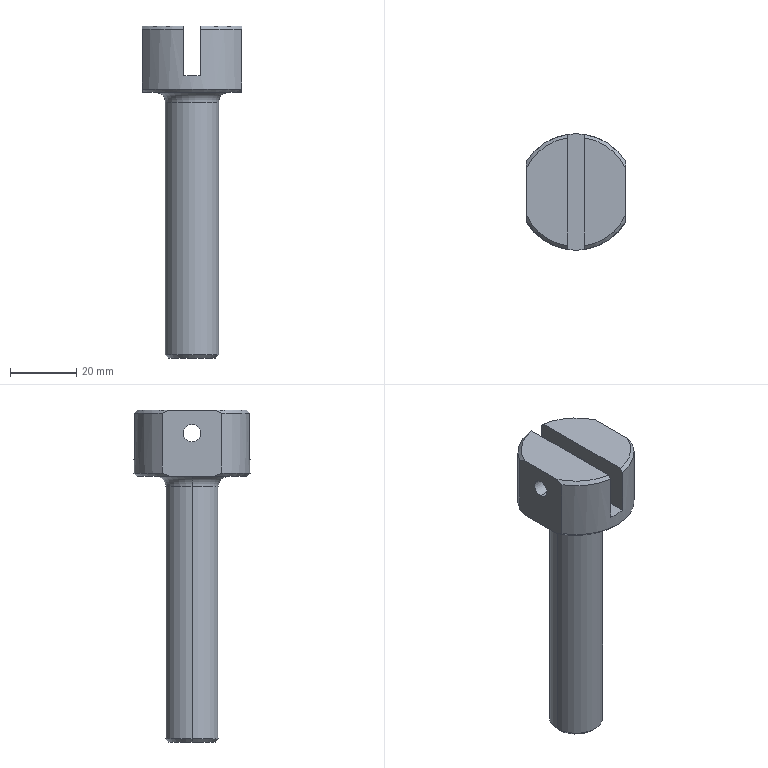Part | SolidWorks | features BaseBody 1 | 1 solid | 27 faces | box 30 x 35 x 100 mm | volume 30973 mm3 | plane 9 | cylinder 8 | cone 8 | torus 2 | commonest cylinder face diameters 5.2 x4 16 x2 35 x2
STEP:
#1=CARTESIAN_POINT('',(-2.5,0.,95.6));
#2=VERTEX_POINT('',#1);
#3=CARTESIAN_POINT('',(-2.5,0.,90.4));
#4=VERTEX_POINT('',#3);
#5=CARTESIAN_POINT('',(-2.5,0.,93.));
#6=DIRECTION('',(1.,0.,0.));
#7=DIRECTION('',(0.,-1.,0.));
#8=AXIS2_PLACEMENT_3D('',#5,#6,#7);
#9=CIRCLE('',#8,2.6);
#10=EDGE_CURVE('',#2,#4,#9,.T.);
#11=ORIENTED_EDGE('',*,*,#10,.T.);
#12=CARTESIAN_POINT('',(-15.,0.,90.4));
#13=VERTEX_POINT('',#12);
#14=CARTESIAN_POINT('',(-15.,0.,90.4));
#15=DIRECTION('',(-1.,0.,0.));
#16=VECTOR('',#15,1000.);
#17=LINE('',#14,#16);
#18=EDGE_CURVE('',#4,#13,#17,.T.);
#19=ORIENTED_EDGE('',*,*,#18,.T.);
#20=CARTESIAN_POINT('',(-15.,0.,95.6));
#21=VERTEX_POINT('',#20);
#22=CARTESIAN_POINT('',(-15.,0.,93.));
#23=DIRECTION('',(-1.,0.,0.));
#24=DIRECTION('',(0.,0.,1.));
#25=AXIS2_PLACEMENT_3D('',#22,#23,#24);
#26=CIRCLE('',#25,2.6);
#27=EDGE_CURVE('',#13,#21,#26,.T.);
#28=ORIENTED_EDGE('',*,*,#27,.T.);
#29=CARTESIAN_POINT('',(-15.,0.,95.6));
#30=DIRECTION('',(-1.,0.,0.));
#31=VECTOR('',#30,1000.);
#32=LINE('',#29,#31);
#33=EDGE_CURVE('',#2,#21,#32,.T.);
#34=ORIENTED_EDGE('',*,*,#33,.F.);
#35=EDGE_LOOP('',(#11,#19,#28,#34));
#36=FACE_OUTER_BOUND('',#35,.T.);
#37=CARTESIAN_POINT('',(-15.,0.,93.));
#38=DIRECTION('',(-1.,0.,0.));
#39=DIRECTION('',(0.,0.,1.));
#40=AXIS2_PLACEMENT_3D('',#37,#38,#39);
#41=CYLINDRICAL_SURFACE('',#40,2.6);
#42=ADVANCED_FACE('',(#36),#41,.F.);
#43=CARTESIAN_POINT('',(-7.,0.,0.));
#44=VERTEX_POINT('',#43);
#45=CARTESIAN_POINT('',(7.,0.,0.));
#46=VERTEX_POINT('',#45);
#47=CARTESIAN_POINT('',(0.,0.,0.));
#48=DIRECTION('',(0.,0.,-1.));
#49=DIRECTION('',(1.,0.,0.));
#50=AXIS2_PLACEMENT_3D('',#47,#48,#49);
#51=CIRCLE('',#50,7.);
#52=EDGE_CURVE('',#44,#46,#51,.T.);
#53=ORIENTED_EDGE('',*,*,#52,.F.);
#54=CARTESIAN_POINT('',(-8.,0.,1.));
#55=VERTEX_POINT('',#54);
#56=CARTESIAN_POINT('',(-8.,0.,1.));
#57=DIRECTION('',(-0.7071,0.,0.7071));
#58=VECTOR('',#57,1000.);
#59=LINE('',#56,#58);
#60=EDGE_CURVE('',#44,#55,#59,.T.);
#61=ORIENTED_EDGE('',*,*,#60,.T.);
#62=CARTESIAN_POINT('',(8.,0.,1.));
#63=VERTEX_POINT('',#62);
#64=CARTESIAN_POINT('',(0.,0.,1.));
#65=DIRECTION('',(0.,0.,1.));
#66=DIRECTION('',(1.,0.,0.));
#67=AXIS2_PLACEMENT_3D('',#64,#65,#66);
#68=CIRCLE('',#67,8.);
#69=EDGE_CURVE('',#63,#55,#68,.T.);
#70=ORIENTED_EDGE('',*,*,#69,.F.);
#71=CARTESIAN_POINT('',(8.,0.,1.));
#72=DIRECTION('',(0.7071,0.,0.7071));
#73=VECTOR('',#72,1000.);
#74=LINE('',#71,#73);
#75=EDGE_CURVE('',#46,#63,#74,.T.);
#76=ORIENTED_EDGE('',*,*,#75,.F.);
#77=EDGE_LOOP('',(#53,#61,#70,#76));
#78=FACE_OUTER_BOUND('',#77,.T.);
#79=CARTESIAN_POINT('',(0.,0.,1.));
#80=DIRECTION('',(0.,0.,1.));
#81=DIRECTION('',(1.,0.,0.));
#82=AXIS2_PLACEMENT_3D('',#79,#80,#81);
#83=CONICAL_SURFACE('',#82,8.,0.7854);
#84=ADVANCED_FACE('',(#78),#83,.T.);
#85=CARTESIAN_POINT('',(-11.,0.,80.));
#86=VERTEX_POINT('',#85);
#87=CARTESIAN_POINT('',(11.,0.,80.));
#88=VERTEX_POINT('',#87);
#89=CARTESIAN_POINT('',(0.,0.,80.));
#90=DIRECTION('',(0.,0.,1.));
#91=DIRECTION('',(1.,0.,0.));
#92=AXIS2_PLACEMENT_3D('',#89,#90,#91);
#93=CIRCLE('',#92,11.);
#94=EDGE_CURVE('',#86,#88,#93,.T.);
#95=ORIENTED_EDGE('',*,*,#94,.F.);
#96=CARTESIAN_POINT('',(-8.,0.,77.));
#97=VERTEX_POINT('',#96);
#98=CARTESIAN_POINT('',(-11.,0.,77.));
#99=DIRECTION('',(0.,1.,0.));
#100=DIRECTION('',(-1.,0.,0.));
#101=AXIS2_PLACEMENT_3D('',#98,#99,#100);
#102=CIRCLE('',#101,3.);
#103=EDGE_CURVE('',#86,#97,#102,.T.);
#104=ORIENTED_EDGE('',*,*,#103,.T.);
#105=CARTESIAN_POINT('',(8.,0.,77.));
#106=VERTEX_POINT('',#105);
#107=CARTESIAN_POINT('',(0.,0.,77.));
#108=DIRECTION('',(0.,0.,-1.));
#109=DIRECTION('',(1.,0.,0.));
#110=AXIS2_PLACEMENT_3D('',#107,#108,#109);
#111=CIRCLE('',#110,8.);
#112=EDGE_CURVE('',#106,#97,#111,.T.);
#113=ORIENTED_EDGE('',*,*,#112,.F.);
#114=CARTESIAN_POINT('',(11.,0.,77.));
#115=DIRECTION('',(0.,-1.,0.));
#116=DIRECTION('',(0.,0.,-1.));
#117=AXIS2_PLACEMENT_3D('',#114,#115,#116);
#118=CIRCLE('',#117,3.);
#119=EDGE_CURVE('',#88,#106,#118,.T.);
#120=ORIENTED_EDGE('',*,*,#119,.F.);
#121=EDGE_LOOP('',(#95,#104,#113,#120));
#122=FACE_OUTER_BOUND('',#121,.T.);
#123=CARTESIAN_POINT('',(0.,0.,77.));
#124=DIRECTION('',(0.,0.,1.));
#125=DIRECTION('',(1.,0.,0.));
#126=AXIS2_PLACEMENT_3D('',#123,#124,#125);
#127=TOROIDAL_SURFACE('',#126,11.,3.);
#128=ADVANCED_FACE('',(#122),#127,.F.);
#129=CARTESIAN_POINT('',(0.,0.,77.));
#130=DIRECTION('',(0.,0.,-1.));
#131=DIRECTION('',(1.,0.,0.));
#132=AXIS2_PLACEMENT_3D('',#129,#130,#131);
#133=CIRCLE('',#132,8.);
#134=EDGE_CURVE('',#97,#106,#133,.T.);
#135=ORIENTED_EDGE('',*,*,#134,.T.);
#136=CARTESIAN_POINT('',(8.,0.,80.));
#137=DIRECTION('',(0.,0.,-1.));
#138=VECTOR('',#137,1000.);
#139=LINE('',#136,#138);
#140=EDGE_CURVE('',#106,#63,#139,.T.);
#141=ORIENTED_EDGE('',*,*,#140,.T.);
#142=ORIENTED_EDGE('',*,*,#69,.T.);
#143=CARTESIAN_POINT('',(-8.,0.,80.));
#144=DIRECTION('',(0.,0.,-1.));
#145=VECTOR('',#144,1000.);
#146=LINE('',#143,#145);
#147=EDGE_CURVE('',#97,#55,#146,.T.);
#148=ORIENTED_EDGE('',*,*,#147,.F.);
#149=EDGE_LOOP('',(#135,#141,#142,#148));
#150=FACE_OUTER_BOUND('',#149,.T.);
#151=CARTESIAN_POINT('',(0.,0.,80.));
#152=DIRECTION('',(0.,0.,-1.));
#153=DIRECTION('',(-1.,0.,0.));
#154=AXIS2_PLACEMENT_3D('',#151,#152,#153);
#155=CYLINDRICAL_SURFACE('',#154,8.);
#156=ADVANCED_FACE('',(#150),#155,.T.);
#157=CARTESIAN_POINT('',(15.,0.,90.4));
#158=VERTEX_POINT('',#157);
#159=CARTESIAN_POINT('',(15.,0.,95.6));
#160=VERTEX_POINT('',#159);
#161=CARTESIAN_POINT('',(15.,0.,93.));
#162=DIRECTION('',(-1.,0.,0.));
#163=DIRECTION('',(0.,0.,1.));
#164=AXIS2_PLACEMENT_3D('',#161,#162,#163);
#165=CIRCLE('',#164,2.6);
#166=EDGE_CURVE('',#158,#160,#165,.T.);
#167=ORIENTED_EDGE('',*,*,#166,.F.);
#168=CARTESIAN_POINT('',(2.5,0.,90.4));
#169=VERTEX_POINT('',#168);
#170=CARTESIAN_POINT('',(-15.,0.,90.4));
#171=DIRECTION('',(-1.,0.,0.));
#172=VECTOR('',#171,1000.);
#173=LINE('',#170,#172);
#174=EDGE_CURVE('',#158,#169,#173,.T.);
#175=ORIENTED_EDGE('',*,*,#174,.T.);
#176=CARTESIAN_POINT('',(2.5,0.,95.6));
#177=VERTEX_POINT('',#176);
#178=CARTESIAN_POINT('',(2.5,0.,93.));
#179=DIRECTION('',(-1.,0.,0.));
#180=DIRECTION('',(0.,1.,0.));
#181=AXIS2_PLACEMENT_3D('',#178,#179,#180);
#182=CIRCLE('',#181,2.6);
#183=EDGE_CURVE('',#169,#177,#182,.T.);
#184=ORIENTED_EDGE('',*,*,#183,.T.);
#185=CARTESIAN_POINT('',(-15.,0.,95.6));
#186=DIRECTION('',(-1.,0.,0.));
#187=VECTOR('',#186,1000.);
#188=LINE('',#185,#187);
#189=EDGE_CURVE('',#160,#177,#188,.T.);
#190=ORIENTED_EDGE('',*,*,#189,.F.);
#191=EDGE_LOOP('',(#167,#175,#184,#190));
#192=FACE_OUTER_BOUND('',#191,.T.);
#193=CARTESIAN_POINT('',(-15.,0.,93.));
#194=DIRECTION('',(-1.,0.,0.));
#195=DIRECTION('',(0.,0.,1.));
#196=AXIS2_PLACEMENT_3D('',#193,#194,#195);
#197=CYLINDRICAL_SURFACE('',#196,2.6);
#198=ADVANCED_FACE('',(#192),#197,.F.);
#199=CARTESIAN_POINT('',(2.5,16.31,100.));
#200=VERTEX_POINT('',#199);
#201=CARTESIAN_POINT('',(2.5,17.321,99.));
#202=VERTEX_POINT('',#201);
#203=CARTESIAN_POINT('',(2.5,16.31,100.));
#204=CARTESIAN_POINT('',(2.5,16.647,99.667));
#205=CARTESIAN_POINT('',(2.5,16.984,99.333));
#206=CARTESIAN_POINT('',(2.5,17.321,99.));
#207=B_SPLINE_CURVE_WITH_KNOTS('',3,(#203,#204,#205,#206),.UNSPECIFIED.,.F.,.F.,(4,4),(0.01912,0.02054),.UNSPECIFIED.);
#208=EDGE_CURVE('',#200,#202,#207,.T.);
#209=ORIENTED_EDGE('',*,*,#208,.F.);
#210=CARTESIAN_POINT('',(15.,6.874,100.));
#211=VERTEX_POINT('',#210);
#212=CARTESIAN_POINT('',(0.,0.,100.));
#213=DIRECTION('',(0.,0.,1.));
#214=DIRECTION('',(1.,0.,0.));
#215=AXIS2_PLACEMENT_3D('',#212,#213,#214);
#216=CIRCLE('',#215,16.5);
#217=EDGE_CURVE('',#211,#200,#216,.T.);
#218=ORIENTED_EDGE('',*,*,#217,.F.);
#219=CARTESIAN_POINT('',(15.,9.014,99.));
#220=VERTEX_POINT('',#219);
#221=CARTESIAN_POINT('',(15.,9.014,99.));
#222=CARTESIAN_POINT('',(15.,8.312,99.362));
#223=CARTESIAN_POINT('',(15.,7.599,99.698));
#224=CARTESIAN_POINT('',(15.,6.874,100.));
#225=B_SPLINE_CURVE_WITH_KNOTS('',3,(#221,#222,#223,#224),.UNSPECIFIED.,.F.,.F.,(4,4),(0.01311,0.01546),.UNSPECIFIED.);
#226=EDGE_CURVE('',#220,#211,#225,.T.);
#227=ORIENTED_EDGE('',*,*,#226,.F.);
#228=CARTESIAN_POINT('',(0.,0.,99.));
#229=DIRECTION('',(0.,0.,-1.));
#230=DIRECTION('',(1.,0.,0.));
#231=AXIS2_PLACEMENT_3D('',#228,#229,#230);
#232=CIRCLE('',#231,17.5);
#233=EDGE_CURVE('',#202,#220,#232,.T.);
#234=ORIENTED_EDGE('',*,*,#233,.F.);
#235=EDGE_LOOP('',(#209,#218,#227,#234));
#236=FACE_OUTER_BOUND('',#235,.T.);
#237=CARTESIAN_POINT('',(0.,0.,100.));
#238=DIRECTION('',(0.,0.,-1.));
#239=DIRECTION('',(-1.,0.,0.));
#240=AXIS2_PLACEMENT_3D('',#237,#238,#239);
#241=CONICAL_SURFACE('',#240,16.5,0.7854);
#242=ADVANCED_FACE('',(#236),#241,.T.);
#243=CARTESIAN_POINT('',(2.5,-16.31,100.));
#244=VERTEX_POINT('',#243);
#245=CARTESIAN_POINT('',(2.5,21.611,100.));
#246=DIRECTION('',(0.,1.,0.));
#247=VECTOR('',#246,1000.);
#248=LINE('',#245,#247);
#249=EDGE_CURVE('',#244,#200,#248,.T.);
#250=ORIENTED_EDGE('',*,*,#249,.F.);
#251=CARTESIAN_POINT('',(15.,-6.874,100.));
#252=VERTEX_POINT('',#251);
#253=CARTESIAN_POINT('',(0.,0.,100.));
#254=DIRECTION('',(0.,0.,1.));
#255=DIRECTION('',(1.,0.,0.));
#256=AXIS2_PLACEMENT_3D('',#253,#254,#255);
#257=CIRCLE('',#256,16.5);
#258=EDGE_CURVE('',#244,#252,#257,.T.);
#259=ORIENTED_EDGE('',*,*,#258,.T.);
#260=CARTESIAN_POINT('',(15.,9.014,100.));
#261=DIRECTION('',(0.,-1.,0.));
#262=VECTOR('',#261,1000.);
#263=LINE('',#260,#262);
#264=EDGE_CURVE('',#211,#252,#263,.T.);
#265=ORIENTED_EDGE('',*,*,#264,.F.);
#266=ORIENTED_EDGE('',*,*,#217,.T.);
#267=EDGE_LOOP('',(#250,#259,#265,#266));
#268=FACE_OUTER_BOUND('',#267,.T.);
#269=CARTESIAN_POINT('',(0.,0.,100.));
#270=DIRECTION('',(0.,0.,1.));
#271=DIRECTION('',(1.,0.,0.));
#272=AXIS2_PLACEMENT_3D('',#269,#270,#271);
#273=PLANE('',#272);
#274=ADVANCED_FACE('',(#268),#273,.T.);
#275=CARTESIAN_POINT('',(2.5,-17.321,99.));
#276=VERTEX_POINT('',#275);
#277=CARTESIAN_POINT('',(2.5,-17.321,99.));
#278=CARTESIAN_POINT('',(2.5,-16.984,99.333));
#279=CARTESIAN_POINT('',(2.5,-16.647,99.667));
#280=CARTESIAN_POINT('',(2.5,-16.31,100.));
#281=B_SPLINE_CURVE_WITH_KNOTS('',3,(#277,#278,#279,#280),.UNSPECIFIED.,.F.,.F.,(4,4),(0.01819,0.01961),.UNSPECIFIED.);
#282=EDGE_CURVE('',#276,#244,#281,.T.);
#283=ORIENTED_EDGE('',*,*,#282,.F.);
#284=CARTESIAN_POINT('',(15.,-9.014,99.));
#285=VERTEX_POINT('',#284);
#286=CARTESIAN_POINT('',(0.,0.,99.));
#287=DIRECTION('',(0.,0.,-1.));
#288=DIRECTION('',(1.,0.,0.));
#289=AXIS2_PLACEMENT_3D('',#286,#287,#288);
#290=CIRCLE('',#289,17.5);
#291=EDGE_CURVE('',#285,#276,#290,.T.);
#292=ORIENTED_EDGE('',*,*,#291,.F.);
#293=CARTESIAN_POINT('',(15.,-6.874,100.));
#294=CARTESIAN_POINT('',(15.,-7.598,99.698));
#295=CARTESIAN_POINT('',(15.,-8.313,99.361));
#296=CARTESIAN_POINT('',(15.,-9.014,99.));
#297=B_SPLINE_CURVE_WITH_KNOTS('',3,(#293,#294,#295,#296),.UNSPECIFIED.,.F.,.F.,(4,4),(0.02959,0.03195),.UNSPECIFIED.);
#298=EDGE_CURVE('',#252,#285,#297,.T.);
#299=ORIENTED_EDGE('',*,*,#298,.F.);
#300=ORIENTED_EDGE('',*,*,#258,.F.);
#301=EDGE_LOOP('',(#283,#292,#299,#300));
#302=FACE_OUTER_BOUND('',#301,.T.);
#303=CARTESIAN_POINT('',(0.,0.,100.));
#304=DIRECTION('',(0.,0.,-1.));
#305=DIRECTION('',(-1.,0.,0.));
#306=AXIS2_PLACEMENT_3D('',#303,#304,#305);
#307=CONICAL_SURFACE('',#306,16.5,0.7854);
#308=ADVANCED_FACE('',(#302),#307,.T.);
#309=ORIENTED_EDGE('',*,*,#174,.F.);
#310=CARTESIAN_POINT('',(15.,0.,93.));
#311=DIRECTION('',(-1.,0.,0.));
#312=DIRECTION('',(0.,0.,1.));
#313=AXIS2_PLACEMENT_3D('',#310,#311,#312);
#314=CIRCLE('',#313,2.6);
#315=EDGE_CURVE('',#160,#158,#314,.T.);
#316=ORIENTED_EDGE('',*,*,#315,.F.);
#317=ORIENTED_EDGE('',*,*,#189,.T.);
#318=CARTESIAN_POINT('',(2.5,0.,93.));
#319=DIRECTION('',(-1.,0.,0.));
#320=DIRECTION('',(0.,1.,0.));
#321=AXIS2_PLACEMENT_3D('',#318,#319,#320);
#322=CIRCLE('',#321,2.6);
#323=EDGE_CURVE('',#177,#169,#322,.T.);
#324=ORIENTED_EDGE('',*,*,#323,.T.);
#325=EDGE_LOOP('',(#309,#316,#317,#324));
#326=FACE_OUTER_BOUND('',#325,.T.);
#327=CARTESIAN_POINT('',(-15.,0.,93.));
#328=DIRECTION('',(-1.,0.,0.));
#329=DIRECTION('',(0.,0.,1.));
#330=AXIS2_PLACEMENT_3D('',#327,#328,#329);
#331=CYLINDRICAL_SURFACE('',#330,2.6);
#332=ADVANCED_FACE('',(#326),#331,.F.);
#333=CARTESIAN_POINT('',(-15.,-9.014,99.));
#334=VERTEX_POINT('',#333);
#335=CARTESIAN_POINT('',(-15.,-6.874,100.));
#336=VERTEX_POINT('',#335);
#337=CARTESIAN_POINT('',(-15.,-9.014,99.));
#338=CARTESIAN_POINT('',(-15.,-8.312,99.362));
#339=CARTESIAN_POINT('',(-15.,-7.599,99.698));
#340=CARTESIAN_POINT('',(-15.,-6.874,100.));
#341=B_SPLINE_CURVE_WITH_KNOTS('',3,(#337,#338,#339,#340),.UNSPECIFIED.,.F.,.F.,(4,4),(0.01311,0.01546),.UNSPECIFIED.);
#342=EDGE_CURVE('',#334,#336,#341,.T.);
#343=ORIENTED_EDGE('',*,*,#342,.T.);
#344=CARTESIAN_POINT('',(-15.,6.874,100.));
#345=VERTEX_POINT('',#344);
#346=CARTESIAN_POINT('',(-15.,9.014,100.));
#347=DIRECTION('',(0.,1.,0.));
#348=VECTOR('',#347,1000.);
#349=LINE('',#346,#348);
#350=EDGE_CURVE('',#336,#345,#349,.T.);
#351=ORIENTED_EDGE('',*,*,#350,.T.);
#352=CARTESIAN_POINT('',(-15.,9.014,99.));
#353=VERTEX_POINT('',#352);
#354=CARTESIAN_POINT('',(-15.,6.874,100.));
#355=CARTESIAN_POINT('',(-15.,7.598,99.698));
#356=CARTESIAN_POINT('',(-15.,8.313,99.361));
#357=CARTESIAN_POINT('',(-15.,9.014,99.));
#358=B_SPLINE_CURVE_WITH_KNOTS('',3,(#354,#355,#356,#357),.UNSPECIFIED.,.F.,.F.,(4,4),(0.02959,0.03195),.UNSPECIFIED.);
#359=EDGE_CURVE('',#345,#353,#358,.T.);
#360=ORIENTED_EDGE('',*,*,#359,.T.);
#361=CARTESIAN_POINT('',(-15.,9.014,81.));
#362=VERTEX_POINT('',#361);
#363=CARTESIAN_POINT('',(-15.,9.014,80.));
#364=DIRECTION('',(0.,0.,1.));
#365=VECTOR('',#364,1000.);
#366=LINE('',#363,#365);
#367=EDGE_CURVE('',#362,#353,#366,.T.);
#368=ORIENTED_EDGE('',*,*,#367,.F.);
#369=CARTESIAN_POINT('',(-15.,6.874,80.));
#370=VERTEX_POINT('',#369);
#371=CARTESIAN_POINT('',(-15.,9.014,81.));
#372=CARTESIAN_POINT('',(-15.,8.312,80.638));
#373=CARTESIAN_POINT('',(-15.,7.599,80.302));
#374=CARTESIAN_POINT('',(-15.,6.874,80.));
#375=B_SPLINE_CURVE_WITH_KNOTS('',3,(#371,#372,#373,#374),.UNSPECIFIED.,.F.,.F.,(4,4),(0.01311,0.01546),.UNSPECIFIED.);
#376=EDGE_CURVE('',#362,#370,#375,.T.);
#377=ORIENTED_EDGE('',*,*,#376,.T.);
#378=CARTESIAN_POINT('',(-15.,-6.874,80.));
#379=VERTEX_POINT('',#378);
#380=CARTESIAN_POINT('',(-15.,9.014,80.));
#381=DIRECTION('',(0.,1.,0.));
#382=VECTOR('',#381,1000.);
#383=LINE('',#380,#382);
#384=EDGE_CURVE('',#379,#370,#383,.T.);
#385=ORIENTED_EDGE('',*,*,#384,.F.);
#386=CARTESIAN_POINT('',(-15.,-9.014,81.));
#387=VERTEX_POINT('',#386);
#388=CARTESIAN_POINT('',(-15.,-6.874,80.));
#389=CARTESIAN_POINT('',(-15.,-7.598,80.302));
#390=CARTESIAN_POINT('',(-15.,-8.313,80.639));
#391=CARTESIAN_POINT('',(-15.,-9.014,81.));
#392=B_SPLINE_CURVE_WITH_KNOTS('',3,(#388,#389,#390,#391),.UNSPECIFIED.,.F.,.F.,(4,4),(0.02959,0.03195),.UNSPECIFIED.);
#393=EDGE_CURVE('',#379,#387,#392,.T.);
#394=ORIENTED_EDGE('',*,*,#393,.T.);
#395=CARTESIAN_POINT('',(-15.,-9.014,80.));
#396=DIRECTION('',(0.,0.,1.));
#397=VECTOR('',#396,1000.);
#398=LINE('',#395,#397);
#399=EDGE_CURVE('',#387,#334,#398,.T.);
#400=ORIENTED_EDGE('',*,*,#399,.T.);
#401=EDGE_LOOP('',(#343,#351,#360,#368,#377,#385,#394,#400));
#402=FACE_OUTER_BOUND('',#401,.T.);
#403=CARTESIAN_POINT('',(-15.,0.,93.));
#404=DIRECTION('',(-1.,0.,0.));
#405=DIRECTION('',(0.,0.,1.));
#406=AXIS2_PLACEMENT_3D('',#403,#404,#405);
#407=CIRCLE('',#406,2.6);
#408=EDGE_CURVE('',#21,#13,#407,.T.);
#409=ORIENTED_EDGE('',*,*,#408,.F.);
#410=ORIENTED_EDGE('',*,*,#27,.F.);
#411=EDGE_LOOP('',(#409,#410));
#412=FACE_BOUND('',#411,.T.);
#413=CARTESIAN_POINT('',(-15.,9.014,80.));
#414=DIRECTION('',(1.,0.,0.));
#415=DIRECTION('',(0.,0.,-1.));
#416=AXIS2_PLACEMENT_3D('',#413,#414,#415);
#417=PLANE('',#416);
#418=ADVANCED_FACE('',(#402,#412),#417,.F.);
#419=CARTESIAN_POINT('',(2.5,17.321,85.));
#420=VERTEX_POINT('',#419);
#421=CARTESIAN_POINT('',(-2.5,17.321,85.));
#422=VERTEX_POINT('',#421);
#423=CARTESIAN_POINT('',(0.,0.,85.));
#424=DIRECTION('',(0.,0.,1.));
#425=DIRECTION('',(1.,0.,0.));
#426=AXIS2_PLACEMENT_3D('',#423,#424,#425);
#427=CIRCLE('',#426,17.5);
#428=EDGE_CURVE('',#420,#422,#427,.T.);
#429=ORIENTED_EDGE('',*,*,#428,.F.);
#430=CARTESIAN_POINT('',(2.5,17.321,100.));
#431=DIRECTION('',(0.,0.,1.));
#432=VECTOR('',#431,1000.);
#433=LINE('',#430,#432);
#434=EDGE_CURVE('',#420,#202,#433,.T.);
#435=ORIENTED_EDGE('',*,*,#434,.T.);
#436=ORIENTED_EDGE('',*,*,#233,.T.);
#437=CARTESIAN_POINT('',(15.,9.014,81.));
#438=VERTEX_POINT('',#437);
#439=CARTESIAN_POINT('',(15.,9.014,80.));
#440=DIRECTION('',(0.,0.,1.));
#441=VECTOR('',#440,1000.);
#442=LINE('',#439,#441);
#443=EDGE_CURVE('',#438,#220,#442,.T.);
#444=ORIENTED_EDGE('',*,*,#443,.F.);
#445=CARTESIAN_POINT('',(0.,0.,81.));
#446=DIRECTION('',(0.,0.,1.));
#447=DIRECTION('',(1.,0.,0.));
#448=AXIS2_PLACEMENT_3D('',#445,#446,#447);
#449=CIRCLE('',#448,17.5);
#450=EDGE_CURVE('',#438,#362,#449,.T.);
#451=ORIENTED_EDGE('',*,*,#450,.T.);
#452=ORIENTED_EDGE('',*,*,#367,.T.);
#453=CARTESIAN_POINT('',(-2.5,17.321,99.));
#454=VERTEX_POINT('',#453);
#455=CARTESIAN_POINT('',(0.,0.,99.));
#456=DIRECTION('',(0.,0.,-1.));
#457=DIRECTION('',(1.,0.,0.));
#458=AXIS2_PLACEMENT_3D('',#455,#456,#457);
#459=CIRCLE('',#458,17.5);
#460=EDGE_CURVE('',#353,#454,#459,.T.);
#461=ORIENTED_EDGE('',*,*,#460,.T.);
#462=CARTESIAN_POINT('',(-2.5,17.321,100.));
#463=DIRECTION('',(0.,0.,-1.));
#464=VECTOR('',#463,1000.);
#465=LINE('',#462,#464);
#466=EDGE_CURVE('',#454,#422,#465,.T.);
#467=ORIENTED_EDGE('',*,*,#466,.T.);
#468=EDGE_LOOP('',(#429,#435,#436,#444,#451,#452,#461,#467));
#469=FACE_OUTER_BOUND('',#468,.T.);
#470=CARTESIAN_POINT('',(0.,0.,100.));
#471=DIRECTION('',(0.,0.,-1.));
#472=DIRECTION('',(-1.,0.,0.));
#473=AXIS2_PLACEMENT_3D('',#470,#471,#472);
#474=CYLINDRICAL_SURFACE('',#473,17.5);
#475=ADVANCED_FACE('',(#469),#474,.T.);
#476=CARTESIAN_POINT('',(-2.5,16.31,100.));
#477=VERTEX_POINT('',#476);
#478=CARTESIAN_POINT('',(-2.5,17.321,99.));
#479=CARTESIAN_POINT('',(-2.5,16.984,99.333));
#480=CARTESIAN_POINT('',(-2.5,16.647,99.667));
#481=CARTESIAN_POINT('',(-2.5,16.31,100.));
#482=B_SPLINE_CURVE_WITH_KNOTS('',3,(#478,#479,#480,#481),.UNSPECIFIED.,.F.,.F.,(4,4),(0.01819,0.01961),.UNSPECIFIED.);
#483=EDGE_CURVE('',#454,#477,#482,.T.);
#484=ORIENTED_EDGE('',*,*,#483,.F.);
#485=ORIENTED_EDGE('',*,*,#460,.F.);
#486=ORIENTED_EDGE('',*,*,#359,.F.);
#487=CARTESIAN_POINT('',(0.,0.,100.));
#488=DIRECTION('',(0.,0.,1.));
#489=DIRECTION('',(1.,0.,0.));
#490=AXIS2_PLACEMENT_3D('',#487,#488,#489);
#491=CIRCLE('',#490,16.5);
#492=EDGE_CURVE('',#477,#345,#491,.T.);
#493=ORIENTED_EDGE('',*,*,#492,.F.);
#494=EDGE_LOOP('',(#484,#485,#486,#493));
#495=FACE_OUTER_BOUND('',#494,.T.);
#496=CARTESIAN_POINT('',(0.,0.,100.));
#497=DIRECTION('',(0.,0.,-1.));
#498=DIRECTION('',(-1.,0.,0.));
#499=AXIS2_PLACEMENT_3D('',#496,#497,#498);
#500=CONICAL_SURFACE('',#499,16.5,0.7854);
#501=ADVANCED_FACE('',(#495),#500,.T.);
#502=CARTESIAN_POINT('',(15.,-9.014,81.));
#503=VERTEX_POINT('',#502);
#504=CARTESIAN_POINT('',(15.,-6.874,80.));
#505=VERTEX_POINT('',#504);
#506=CARTESIAN_POINT('',(15.,-9.014,81.));
#507=CARTESIAN_POINT('',(15.,-8.312,80.638));
#508=CARTESIAN_POINT('',(15.,-7.599,80.302));
#509=CARTESIAN_POINT('',(15.,-6.874,80.));
#510=B_SPLINE_CURVE_WITH_KNOTS('',3,(#506,#507,#508,#509),.UNSPECIFIED.,.F.,.F.,(4,4),(0.01311,0.01546),.UNSPECIFIED.);
#511=EDGE_CURVE('',#503,#505,#510,.T.);
#512=ORIENTED_EDGE('',*,*,#511,.F.);
#513=CARTESIAN_POINT('',(0.,0.,81.));
#514=DIRECTION('',(0.,0.,1.));
#515=DIRECTION('',(1.,0.,0.));
#516=AXIS2_PLACEMENT_3D('',#513,#514,#515);
#517=CIRCLE('',#516,17.5);
#518=EDGE_CURVE('',#387,#503,#517,.T.);
#519=ORIENTED_EDGE('',*,*,#518,.F.);
#520=ORIENTED_EDGE('',*,*,#393,.F.);
#521=CARTESIAN_POINT('',(0.,0.,80.));
#522=DIRECTION('',(0.,0.,-1.));
#523=DIRECTION('',(1.,0.,0.));
#524=AXIS2_PLACEMENT_3D('',#521,#522,#523);
#525=CIRCLE('',#524,16.5);
#526=EDGE_CURVE('',#505,#379,#525,.T.);
#527=ORIENTED_EDGE('',*,*,#526,.F.);
#528=EDGE_LOOP('',(#512,#519,#520,#527));
#529=FACE_OUTER_BOUND('',#528,.T.);
#530=CARTESIAN_POINT('',(0.,0.,81.));
#531=DIRECTION('',(0.,0.,1.));
#532=DIRECTION('',(1.,0.,0.));
#533=AXIS2_PLACEMENT_3D('',#530,#531,#532);
#534=CONICAL_SURFACE('',#533,17.5,0.7854);
#535=ADVANCED_FACE('',(#529),#534,.T.);
#536=ORIENTED_EDGE('',*,*,#140,.F.);
#537=ORIENTED_EDGE('',*,*,#112,.T.);
#538=ORIENTED_EDGE('',*,*,#147,.T.);
#539=CARTESIAN_POINT('',(0.,0.,1.));
#540=DIRECTION('',(0.,0.,1.));
#541=DIRECTION('',(1.,0.,0.));
#542=AXIS2_PLACEMENT_3D('',#539,#540,#541);
#543=CIRCLE('',#542,8.);
#544=EDGE_CURVE('',#55,#63,#543,.T.);
#545=ORIENTED_EDGE('',*,*,#544,.T.);
#546=EDGE_LOOP('',(#536,#537,#538,#545));
#547=FACE_OUTER_BOUND('',#546,.T.);
#548=CARTESIAN_POINT('',(0.,0.,80.));
#549=DIRECTION('',(0.,0.,-1.));
#550=DIRECTION('',(-1.,0.,0.));
#551=AXIS2_PLACEMENT_3D('',#548,#549,#550);
#552=CYLINDRICAL_SURFACE('',#551,8.);
#553=ADVANCED_FACE('',(#547),#552,.T.);
#554=CARTESIAN_POINT('',(0.,0.,0.));
#555=DIRECTION('',(0.,0.,-1.));
#556=DIRECTION('',(1.,0.,0.));
#557=AXIS2_PLACEMENT_3D('',#554,#555,#556);
#558=CIRCLE('',#557,7.);
#559=EDGE_CURVE('',#46,#44,#558,.T.);
#560=ORIENTED_EDGE('',*,*,#559,.T.);
#561=ORIENTED_EDGE('',*,*,#52,.T.);
#562=EDGE_LOOP('',(#560,#561));
#563=FACE_OUTER_BOUND('',#562,.T.);
#564=CARTESIAN_POINT('',(0.,0.,0.));
#565=DIRECTION('',(0.,0.,1.));
#566=DIRECTION('',(1.,0.,0.));
#567=AXIS2_PLACEMENT_3D('',#564,#565,#566);
#568=PLANE('',#567);
#569=ADVANCED_FACE('',(#563),#568,.F.);
#570=ORIENTED_EDGE('',*,*,#291,.T.);
#571=CARTESIAN_POINT('',(2.5,-17.321,85.));
#572=VERTEX_POINT('',#571);
#573=CARTESIAN_POINT('',(2.5,-17.321,100.));
#574=DIRECTION('',(0.,0.,-1.));
#575=VECTOR('',#574,1000.);
#576=LINE('',#573,#575);
#577=EDGE_CURVE('',#276,#572,#576,.T.);
#578=ORIENTED_EDGE('',*,*,#577,.T.);
#579=CARTESIAN_POINT('',(-2.5,-17.321,85.));
#580=VERTEX_POINT('',#579);
#581=CARTESIAN_POINT('',(0.,0.,85.));
#582=DIRECTION('',(0.,0.,1.));
#583=DIRECTION('',(1.,0.,0.));
#584=AXIS2_PLACEMENT_3D('',#581,#582,#583);
#585=CIRCLE('',#584,17.5);
#586=EDGE_CURVE('',#580,#572,#585,.T.);
#587=ORIENTED_EDGE('',*,*,#586,.F.);
#588=CARTESIAN_POINT('',(-2.5,-17.321,99.));
#589=VERTEX_POINT('',#588);
#590=CARTESIAN_POINT('',(-2.5,-17.321,100.));
#591=DIRECTION('',(0.,0.,1.));
#592=VECTOR('',#591,1000.);
#593=LINE('',#590,#592);
#594=EDGE_CURVE('',#580,#589,#593,.T.);
#595=ORIENTED_EDGE('',*,*,#594,.T.);
#596=CARTESIAN_POINT('',(0.,0.,99.));
#597=DIRECTION('',(0.,0.,-1.));
#598=DIRECTION('',(1.,0.,0.));
#599=AXIS2_PLACEMENT_3D('',#596,#597,#598);
#600=CIRCLE('',#599,17.5);
#601=EDGE_CURVE('',#589,#334,#600,.T.);
#602=ORIENTED_EDGE('',*,*,#601,.T.);
#603=ORIENTED_EDGE('',*,*,#399,.F.);
#604=ORIENTED_EDGE('',*,*,#518,.T.);
#605=CARTESIAN_POINT('',(15.,-9.014,80.));
#606=DIRECTION('',(0.,0.,1.));
#607=VECTOR('',#606,1000.);
#608=LINE('',#605,#607);
#609=EDGE_CURVE('',#503,#285,#608,.T.);
#610=ORIENTED_EDGE('',*,*,#609,.T.);
#611=EDGE_LOOP('',(#570,#578,#587,#595,#602,#603,#604,#610));
#612=FACE_OUTER_BOUND('',#611,.T.);
#613=CARTESIAN_POINT('',(0.,0.,100.));
#614=DIRECTION('',(0.,0.,-1.));
#615=DIRECTION('',(-1.,0.,0.));
#616=AXIS2_PLACEMENT_3D('',#613,#614,#615);
#617=CYLINDRICAL_SURFACE('',#616,17.5);
#618=ADVANCED_FACE('',(#612),#617,.T.);
#619=CARTESIAN_POINT('',(-2.5,-16.31,100.));
#620=VERTEX_POINT('',#619);
#621=CARTESIAN_POINT('',(-2.5,21.611,100.));
#622=DIRECTION('',(0.,-1.,0.));
#623=VECTOR('',#622,1000.);
#624=LINE('',#621,#623);
#625=EDGE_CURVE('',#477,#620,#624,.T.);
#626=ORIENTED_EDGE('',*,*,#625,.F.);
#627=ORIENTED_EDGE('',*,*,#492,.T.);
#628=ORIENTED_EDGE('',*,*,#350,.F.);
#629=CARTESIAN_POINT('',(0.,0.,100.));
#630=DIRECTION('',(0.,0.,1.));
#631=DIRECTION('',(1.,0.,0.));
#632=AXIS2_PLACEMENT_3D('',#629,#630,#631);
#633=CIRCLE('',#632,16.5);
#634=EDGE_CURVE('',#336,#620,#633,.T.);
#635=ORIENTED_EDGE('',*,*,#634,.T.);
#636=EDGE_LOOP('',(#626,#627,#628,#635));
#637=FACE_OUTER_BOUND('',#636,.T.);
#638=CARTESIAN_POINT('',(0.,0.,100.));
#639=DIRECTION('',(0.,0.,1.));
#640=DIRECTION('',(1.,0.,0.));
#641=AXIS2_PLACEMENT_3D('',#638,#639,#640);
#642=PLANE('',#641);
#643=ADVANCED_FACE('',(#637),#642,.T.);
#644=CARTESIAN_POINT('',(15.,6.874,80.));
#645=VERTEX_POINT('',#644);
#646=CARTESIAN_POINT('',(0.,0.,80.));
#647=DIRECTION('',(0.,0.,-1.));
#648=DIRECTION('',(1.,0.,0.));
#649=AXIS2_PLACEMENT_3D('',#646,#647,#648);
#650=CIRCLE('',#649,16.5);
#651=EDGE_CURVE('',#370,#645,#650,.T.);
#652=ORIENTED_EDGE('',*,*,#651,.T.);
#653=CARTESIAN_POINT('',(15.,9.014,80.));
#654=DIRECTION('',(0.,-1.,0.));
#655=VECTOR('',#654,1000.);
#656=LINE('',#653,#655);
#657=EDGE_CURVE('',#645,#505,#656,.T.);
#658=ORIENTED_EDGE('',*,*,#657,.T.);
#659=ORIENTED_EDGE('',*,*,#526,.T.);
#660=ORIENTED_EDGE('',*,*,#384,.T.);
#661=EDGE_LOOP('',(#652,#658,#659,#660));
#662=FACE_OUTER_BOUND('',#661,.T.);
#663=CARTESIAN_POINT('',(0.,0.,80.));
#664=DIRECTION('',(0.,0.,1.));
#665=DIRECTION('',(1.,0.,0.));
#666=AXIS2_PLACEMENT_3D('',#663,#664,#665);
#667=CIRCLE('',#666,11.);
#668=EDGE_CURVE('',#88,#86,#667,.T.);
#669=ORIENTED_EDGE('',*,*,#668,.T.);
#670=ORIENTED_EDGE('',*,*,#94,.T.);
#671=EDGE_LOOP('',(#669,#670));
#672=FACE_BOUND('',#671,.T.);
#673=CARTESIAN_POINT('',(0.,0.,80.));
#674=DIRECTION('',(0.,0.,1.));
#675=DIRECTION('',(1.,0.,0.));
#676=AXIS2_PLACEMENT_3D('',#673,#674,#675);
#677=PLANE('',#676);
#678=ADVANCED_FACE('',(#662,#672),#677,.F.);
#679=ORIENTED_EDGE('',*,*,#103,.F.);
#680=ORIENTED_EDGE('',*,*,#668,.F.);
#681=ORIENTED_EDGE('',*,*,#119,.T.);
#682=ORIENTED_EDGE('',*,*,#134,.F.);
#683=EDGE_LOOP('',(#679,#680,#681,#682));
#684=FACE_OUTER_BOUND('',#683,.T.);
#685=CARTESIAN_POINT('',(0.,0.,77.));
#686=DIRECTION('',(0.,0.,1.));
#687=DIRECTION('',(1.,0.,0.));
#688=AXIS2_PLACEMENT_3D('',#685,#686,#687);
#689=TOROIDAL_SURFACE('',#688,11.,3.);
#690=ADVANCED_FACE('',(#684),#689,.F.);
#691=CARTESIAN_POINT('',(-2.5,-16.31,100.));
#692=CARTESIAN_POINT('',(-2.5,-16.647,99.667));
#693=CARTESIAN_POINT('',(-2.5,-16.984,99.333));
#694=CARTESIAN_POINT('',(-2.5,-17.321,99.));
#695=B_SPLINE_CURVE_WITH_KNOTS('',3,(#691,#692,#693,#694),.UNSPECIFIED.,.F.,.F.,(4,4),(0.01912,0.02054),.UNSPECIFIED.);
#696=EDGE_CURVE('',#620,#589,#695,.T.);
#697=ORIENTED_EDGE('',*,*,#696,.F.);
#698=ORIENTED_EDGE('',*,*,#634,.F.);
#699=ORIENTED_EDGE('',*,*,#342,.F.);
#700=ORIENTED_EDGE('',*,*,#601,.F.);
#701=EDGE_LOOP('',(#697,#698,#699,#700));
#702=FACE_OUTER_BOUND('',#701,.T.);
#703=CARTESIAN_POINT('',(0.,0.,100.));
#704=DIRECTION('',(0.,0.,-1.));
#705=DIRECTION('',(-1.,0.,0.));
#706=AXIS2_PLACEMENT_3D('',#703,#704,#705);
#707=CONICAL_SURFACE('',#706,16.5,0.7854);
#708=ADVANCED_FACE('',(#702),#707,.T.);
#709=CARTESIAN_POINT('',(15.,6.874,80.));
#710=CARTESIAN_POINT('',(15.,7.598,80.302));
#711=CARTESIAN_POINT('',(15.,8.313,80.639));
#712=CARTESIAN_POINT('',(15.,9.014,81.));
#713=B_SPLINE_CURVE_WITH_KNOTS('',3,(#709,#710,#711,#712),.UNSPECIFIED.,.F.,.F.,(4,4),(0.02959,0.03195),.UNSPECIFIED.);
#714=EDGE_CURVE('',#645,#438,#713,.T.);
#715=ORIENTED_EDGE('',*,*,#714,.F.);
#716=ORIENTED_EDGE('',*,*,#651,.F.);
#717=ORIENTED_EDGE('',*,*,#376,.F.);
#718=ORIENTED_EDGE('',*,*,#450,.F.);
#719=EDGE_LOOP('',(#715,#716,#717,#718));
#720=FACE_OUTER_BOUND('',#719,.T.);
#721=CARTESIAN_POINT('',(0.,0.,81.));
#722=DIRECTION('',(0.,0.,1.));
#723=DIRECTION('',(1.,0.,0.));
#724=AXIS2_PLACEMENT_3D('',#721,#722,#723);
#725=CONICAL_SURFACE('',#724,17.5,0.7854);
#726=ADVANCED_FACE('',(#720),#725,.T.);
#727=ORIENTED_EDGE('',*,*,#60,.F.);
#728=ORIENTED_EDGE('',*,*,#559,.F.);
#729=ORIENTED_EDGE('',*,*,#75,.T.);
#730=ORIENTED_EDGE('',*,*,#544,.F.);
#731=EDGE_LOOP('',(#727,#728,#729,#730));
#732=FACE_OUTER_BOUND('',#731,.T.);
#733=CARTESIAN_POINT('',(0.,0.,1.));
#734=DIRECTION('',(0.,0.,1.));
#735=DIRECTION('',(1.,0.,0.));
#736=AXIS2_PLACEMENT_3D('',#733,#734,#735);
#737=CONICAL_SURFACE('',#736,8.,0.7854);
#738=ADVANCED_FACE('',(#732),#737,.T.);
#739=ORIENTED_EDGE('',*,*,#315,.T.);
#740=ORIENTED_EDGE('',*,*,#166,.T.);
#741=EDGE_LOOP('',(#739,#740));
#742=FACE_BOUND('',#741,.T.);
#743=ORIENTED_EDGE('',*,*,#226,.T.);
#744=ORIENTED_EDGE('',*,*,#264,.T.);
#745=ORIENTED_EDGE('',*,*,#298,.T.);
#746=ORIENTED_EDGE('',*,*,#609,.F.);
#747=ORIENTED_EDGE('',*,*,#511,.T.);
#748=ORIENTED_EDGE('',*,*,#657,.F.);
#749=ORIENTED_EDGE('',*,*,#714,.T.);
#750=ORIENTED_EDGE('',*,*,#443,.T.);
#751=EDGE_LOOP('',(#743,#744,#745,#746,#747,#748,#749,#750));
#752=FACE_OUTER_BOUND('',#751,.T.);
#753=CARTESIAN_POINT('',(15.,9.014,80.));
#754=DIRECTION('',(-1.,0.,0.));
#755=DIRECTION('',(0.,0.,1.));
#756=AXIS2_PLACEMENT_3D('',#753,#754,#755);
#757=PLANE('',#756);
#758=ADVANCED_FACE('',(#742,#752),#757,.F.);
#759=ORIENTED_EDGE('',*,*,#18,.F.);
#760=CARTESIAN_POINT('',(-2.5,0.,93.));
#761=DIRECTION('',(1.,0.,0.));
#762=DIRECTION('',(0.,-1.,0.));
#763=AXIS2_PLACEMENT_3D('',#760,#761,#762);
#764=CIRCLE('',#763,2.6);
#765=EDGE_CURVE('',#4,#2,#764,.T.);
#766=ORIENTED_EDGE('',*,*,#765,.T.);
#767=ORIENTED_EDGE('',*,*,#33,.T.);
#768=ORIENTED_EDGE('',*,*,#408,.T.);
#769=EDGE_LOOP('',(#759,#766,#767,#768));
#770=FACE_OUTER_BOUND('',#769,.T.);
#771=CARTESIAN_POINT('',(-15.,0.,93.));
#772=DIRECTION('',(-1.,0.,0.));
#773=DIRECTION('',(0.,0.,1.));
#774=AXIS2_PLACEMENT_3D('',#771,#772,#773);
#775=CYLINDRICAL_SURFACE('',#774,2.6);
#776=ADVANCED_FACE('',(#770),#775,.F.);
#777=ORIENTED_EDGE('',*,*,#428,.T.);
#778=CARTESIAN_POINT('',(-2.5,21.611,85.));
#779=DIRECTION('',(0.,-1.,0.));
#780=VECTOR('',#779,1000.);
#781=LINE('',#778,#780);
#782=EDGE_CURVE('',#422,#580,#781,.T.);
#783=ORIENTED_EDGE('',*,*,#782,.T.);
#784=ORIENTED_EDGE('',*,*,#586,.T.);
#785=CARTESIAN_POINT('',(2.5,21.611,85.));
#786=DIRECTION('',(0.,1.,0.));
#787=VECTOR('',#786,1000.);
#788=LINE('',#785,#787);
#789=EDGE_CURVE('',#572,#420,#788,.T.);
#790=ORIENTED_EDGE('',*,*,#789,.T.);
#791=EDGE_LOOP('',(#777,#783,#784,#790));
#792=FACE_OUTER_BOUND('',#791,.T.);
#793=CARTESIAN_POINT('',(0.,0.,85.));
#794=DIRECTION('',(0.,0.,1.));
#795=DIRECTION('',(1.,0.,0.));
#796=AXIS2_PLACEMENT_3D('',#793,#794,#795);
#797=PLANE('',#796);
#798=ADVANCED_FACE('',(#792),#797,.T.);
#799=ORIENTED_EDGE('',*,*,#323,.F.);
#800=ORIENTED_EDGE('',*,*,#183,.F.);
#801=EDGE_LOOP('',(#799,#800));
#802=FACE_BOUND('',#801,.T.);
#803=ORIENTED_EDGE('',*,*,#789,.F.);
#804=ORIENTED_EDGE('',*,*,#577,.F.);
#805=ORIENTED_EDGE('',*,*,#282,.T.);
#806=ORIENTED_EDGE('',*,*,#249,.T.);
#807=ORIENTED_EDGE('',*,*,#208,.T.);
#808=ORIENTED_EDGE('',*,*,#434,.F.);
#809=EDGE_LOOP('',(#803,#804,#805,#806,#807,#808));
#810=FACE_OUTER_BOUND('',#809,.T.);
#811=CARTESIAN_POINT('',(2.5,21.611,85.));
#812=DIRECTION('',(1.,0.,0.));
#813=DIRECTION('',(0.,1.,0.));
#814=AXIS2_PLACEMENT_3D('',#811,#812,#813);
#815=PLANE('',#814);
#816=ADVANCED_FACE('',(#802,#810),#815,.F.);
#817=ORIENTED_EDGE('',*,*,#10,.F.);
#818=ORIENTED_EDGE('',*,*,#765,.F.);
#819=EDGE_LOOP('',(#817,#818));
#820=FACE_BOUND('',#819,.T.);
#821=ORIENTED_EDGE('',*,*,#483,.T.);
#822=ORIENTED_EDGE('',*,*,#625,.T.);
#823=ORIENTED_EDGE('',*,*,#696,.T.);
#824=ORIENTED_EDGE('',*,*,#594,.F.);
#825=ORIENTED_EDGE('',*,*,#782,.F.);
#826=ORIENTED_EDGE('',*,*,#466,.F.);
#827=EDGE_LOOP('',(#821,#822,#823,#824,#825,#826));
#828=FACE_OUTER_BOUND('',#827,.T.);
#829=CARTESIAN_POINT('',(-2.5,21.611,85.));
#830=DIRECTION('',(-1.,0.,0.));
#831=DIRECTION('',(0.,-1.,0.));
#832=AXIS2_PLACEMENT_3D('',#829,#830,#831);
#833=PLANE('',#832);
#834=ADVANCED_FACE('',(#820,#828),#833,.F.);
#835=CLOSED_SHELL('',(#42,#84,#128,#156,#198,#242,#274,#308,#332,#418,#475,#501,#535,#553,#569,#618,#643,#678,#690,#708,#726,#738,#758,#776,#798,#816,#834));
#836=MANIFOLD_SOLID_BREP('',#835);
#837=CARTESIAN_POINT('',(0.,0.,0.));
#838=DIRECTION('',(0.,0.,1.));
#839=DIRECTION('',(1.,0.,0.));
#840=AXIS2_PLACEMENT_3D('',#837,#838,#839);
#841=(LENGTH_UNIT()NAMED_UNIT(*)SI_UNIT(.MILLI.,.METRE.));
#842=UNCERTAINTY_MEASURE_WITH_UNIT(LENGTH_MEASURE(0.00001),#841,'','');
#843=(NAMED_UNIT(*)PLANE_ANGLE_UNIT()SI_UNIT($,.RADIAN.));
#844=(NAMED_UNIT(*)SI_UNIT($,.STERADIAN.)SOLID_ANGLE_UNIT());
#845=(GEOMETRIC_REPRESENTATION_CONTEXT(3)GLOBAL_UNCERTAINTY_ASSIGNED_CONTEXT((#842))GLOBAL_UNIT_ASSIGNED_CONTEXT((#841,#843,#844))REPRESENTATION_CONTEXT('',''));
#846=ADVANCED_BREP_SHAPE_REPRESENTATION('',(#836,#840),#845);